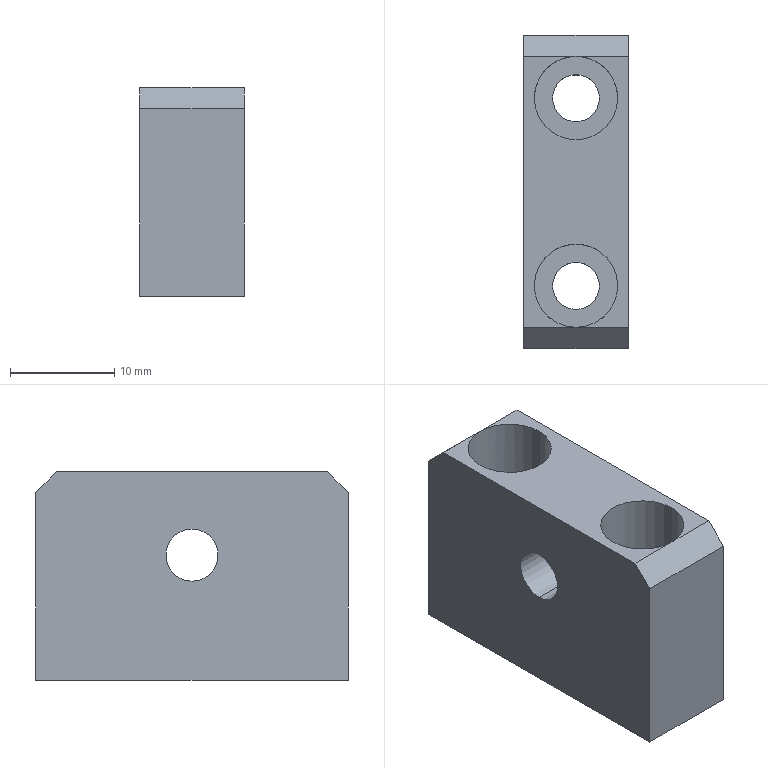Part | STEP file | PN_0029 | 1 solid | 20 faces | box 10 x 30 x 20 mm | volume 4165 mm3 | cylinder 10 | plane 10 | commonest cylinder face diameters 4.5 x4 8 x4 5 x2